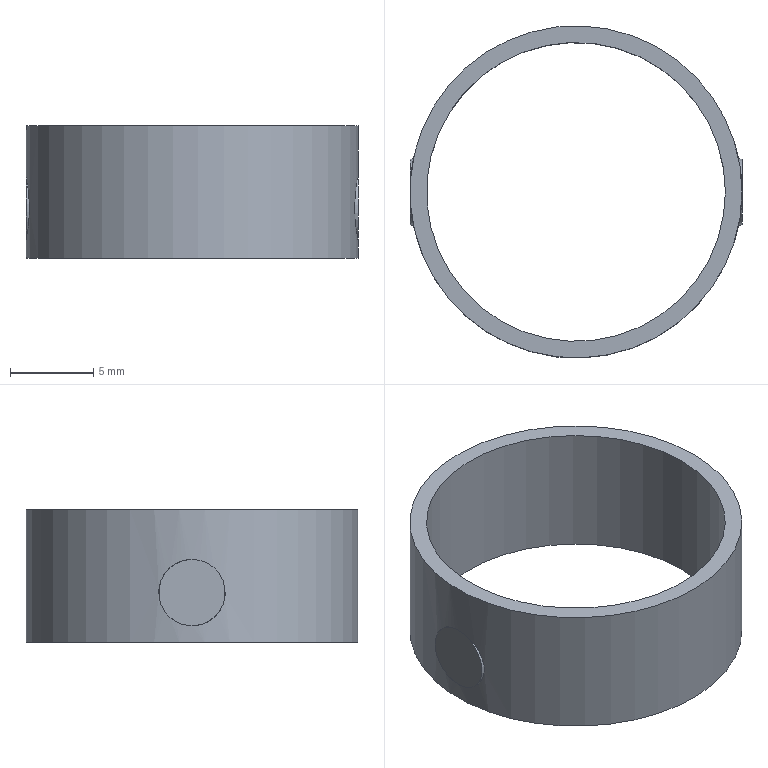Part | NX | features DATUM_CSYS 3, EXTRUDE 2, SKETCH 2, UNITE 2, Container 1, EXTRACT_BODY 1, Geometry Instance 1 | 1 solid | 10 faces | box 20 x 20 x 8 mm | volume 478.886 mm3 | cylinder 6 | plane 4 | commonest cylinder face diameters 4 x4 18 x1 20 x1
STEP:
#1=CARTESIAN_POINT('',(-10.,0.,1.));
#2=VERTEX_POINT('',#1);
#3=CARTESIAN_POINT('',(-10.,0.,5.));
#4=VERTEX_POINT('',#3);
#5=CARTESIAN_POINT('',(-10.,0.,1.));
#6=CARTESIAN_POINT('',(-10.,0.5227,1.));
#7=CARTESIAN_POINT('',(-9.9,1.565,1.432));
#8=CARTESIAN_POINT('',(-9.747,2.217,2.999));
#9=CARTESIAN_POINT('',(-9.9,1.565,4.566));
#10=CARTESIAN_POINT('',(-10.,0.5299,5.));
#11=CARTESIAN_POINT('',(-10.,0.,5.));
#12=B_SPLINE_CURVE_WITH_KNOTS('',3,(#5,#6,#7,#8,#9,#10,#11),.UNSPECIFIED.,.F.,.F.,(4,1,1,1,4),(0.006269,0.007836,0.009402,0.01097,0.01254),.UNSPECIFIED.);
#13=EDGE_CURVE('',#2,#4,#12,.T.);
#14=ORIENTED_EDGE('',*,*,#13,.F.);
#15=CARTESIAN_POINT('',(-10.,0.,3.));
#16=DIRECTION('',(1.,0.,0.));
#17=DIRECTION('',(0.,1.,0.));
#18=AXIS2_PLACEMENT_3D('',#15,#16,#17);
#19=CIRCLE('',#18,2.);
#20=EDGE_CURVE('',#4,#2,#19,.F.);
#21=ORIENTED_EDGE('',*,*,#20,.F.);
#22=EDGE_LOOP('',(#14,#21));
#23=FACE_BOUND('',#22,.T.);
#24=CARTESIAN_POINT('',(-10.,0.,3.));
#25=DIRECTION('',(1.,0.,0.));
#26=DIRECTION('',(0.,0.,1.));
#27=AXIS2_PLACEMENT_3D('',#24,#25,#26);
#28=CYLINDRICAL_SURFACE('',#27,2.);
#29=ADVANCED_FACE('',(#23),#28,.T.);
#30=CARTESIAN_POINT('',(-10.,0.,5.));
#31=CARTESIAN_POINT('',(-10.,-0.53,5.));
#32=CARTESIAN_POINT('',(-9.9,-1.564,4.566));
#33=CARTESIAN_POINT('',(-9.747,-2.217,3.002));
#34=CARTESIAN_POINT('',(-9.9,-1.567,1.432));
#35=CARTESIAN_POINT('',(-10.,-0.5228,1.));
#36=CARTESIAN_POINT('',(-10.,0.,1.));
#37=B_SPLINE_CURVE_WITH_KNOTS('',3,(#30,#31,#32,#33,#34,#35,#36),.UNSPECIFIED.,.F.,.F.,(4,1,1,1,4),(0.,0.001567,0.003134,0.004702,0.006269),.UNSPECIFIED.);
#38=EDGE_CURVE('',#4,#2,#37,.T.);
#39=ORIENTED_EDGE('',*,*,#38,.F.);
#40=CARTESIAN_POINT('',(-10.,0.,3.));
#41=DIRECTION('',(1.,0.,0.));
#42=DIRECTION('',(0.,1.,0.));
#43=AXIS2_PLACEMENT_3D('',#40,#41,#42);
#44=CIRCLE('',#43,2.);
#45=EDGE_CURVE('',#2,#4,#44,.F.);
#46=ORIENTED_EDGE('',*,*,#45,.F.);
#47=EDGE_LOOP('',(#39,#46));
#48=FACE_BOUND('',#47,.T.);
#49=CARTESIAN_POINT('',(-10.,0.,3.));
#50=DIRECTION('',(1.,0.,0.));
#51=DIRECTION('',(0.,0.,1.));
#52=AXIS2_PLACEMENT_3D('',#49,#50,#51);
#53=CYLINDRICAL_SURFACE('',#52,2.);
#54=ADVANCED_FACE('',(#48),#53,.T.);
#55=ORIENTED_EDGE('',*,*,#45,.T.);
#56=ORIENTED_EDGE('',*,*,#20,.T.);
#57=EDGE_LOOP('',(#55,#56));
#58=FACE_BOUND('',#57,.T.);
#59=CARTESIAN_POINT('',(-10.,0.,3.));
#60=DIRECTION('',(-1.,0.,0.));
#61=DIRECTION('',(0.,0.,-1.));
#62=AXIS2_PLACEMENT_3D('',#59,#60,#61);
#63=PLANE('',#62);
#64=ADVANCED_FACE('',(#58),#63,.T.);
#65=CARTESIAN_POINT('',(10.,0.,1.));
#66=VERTEX_POINT('',#65);
#67=CARTESIAN_POINT('',(10.,0.,5.));
#68=VERTEX_POINT('',#67);
#69=CARTESIAN_POINT('',(10.,0.,3.));
#70=DIRECTION('',(1.,0.,0.));
#71=DIRECTION('',(0.,1.,0.));
#72=AXIS2_PLACEMENT_3D('',#69,#70,#71);
#73=CIRCLE('',#72,2.);
#74=EDGE_CURVE('',#66,#68,#73,.T.);
#75=ORIENTED_EDGE('',*,*,#74,.T.);
#76=CARTESIAN_POINT('',(10.,0.,3.));
#77=DIRECTION('',(1.,0.,0.));
#78=DIRECTION('',(0.,1.,0.));
#79=AXIS2_PLACEMENT_3D('',#76,#77,#78);
#80=CIRCLE('',#79,2.);
#81=EDGE_CURVE('',#68,#66,#80,.T.);
#82=ORIENTED_EDGE('',*,*,#81,.T.);
#83=EDGE_LOOP('',(#75,#82));
#84=FACE_BOUND('',#83,.T.);
#85=CARTESIAN_POINT('',(10.,0.,3.));
#86=DIRECTION('',(1.,0.,0.));
#87=DIRECTION('',(0.,0.,-1.));
#88=AXIS2_PLACEMENT_3D('',#85,#86,#87);
#89=PLANE('',#88);
#90=ADVANCED_FACE('',(#84),#89,.T.);
#91=CARTESIAN_POINT('',(10.,0.,5.));
#92=CARTESIAN_POINT('',(10.,0.53,5.));
#93=CARTESIAN_POINT('',(9.9,1.564,4.566));
#94=CARTESIAN_POINT('',(9.747,2.217,3.002));
#95=CARTESIAN_POINT('',(9.9,1.567,1.432));
#96=CARTESIAN_POINT('',(10.,0.5228,1.));
#97=CARTESIAN_POINT('',(10.,0.,1.));
#98=B_SPLINE_CURVE_WITH_KNOTS('',3,(#91,#92,#93,#94,#95,#96,#97),.UNSPECIFIED.,.F.,.F.,(4,1,1,1,4),(0.,0.001567,0.003134,0.004702,0.006269),.UNSPECIFIED.);
#99=EDGE_CURVE('',#68,#66,#98,.T.);
#100=ORIENTED_EDGE('',*,*,#99,.F.);
#101=ORIENTED_EDGE('',*,*,#74,.F.);
#102=EDGE_LOOP('',(#100,#101));
#103=FACE_BOUND('',#102,.T.);
#104=CARTESIAN_POINT('',(10.,0.,3.));
#105=DIRECTION('',(-1.,0.,0.));
#106=DIRECTION('',(0.,0.,1.));
#107=AXIS2_PLACEMENT_3D('',#104,#105,#106);
#108=CYLINDRICAL_SURFACE('',#107,2.);
#109=ADVANCED_FACE('',(#103),#108,.T.);
#110=CARTESIAN_POINT('',(10.,0.,1.));
#111=CARTESIAN_POINT('',(10.,-0.5227,1.));
#112=CARTESIAN_POINT('',(9.9,-1.565,1.432));
#113=CARTESIAN_POINT('',(9.747,-2.217,2.999));
#114=CARTESIAN_POINT('',(9.9,-1.565,4.566));
#115=CARTESIAN_POINT('',(10.,-0.5299,5.));
#116=CARTESIAN_POINT('',(10.,0.,5.));
#117=B_SPLINE_CURVE_WITH_KNOTS('',3,(#110,#111,#112,#113,#114,#115,#116),.UNSPECIFIED.,.F.,.F.,(4,1,1,1,4),(0.006269,0.007836,0.009402,0.01097,0.01254),.UNSPECIFIED.);
#118=EDGE_CURVE('',#66,#68,#117,.T.);
#119=ORIENTED_EDGE('',*,*,#118,.F.);
#120=ORIENTED_EDGE('',*,*,#81,.F.);
#121=EDGE_LOOP('',(#119,#120));
#122=FACE_BOUND('',#121,.T.);
#123=CARTESIAN_POINT('',(10.,0.,3.));
#124=DIRECTION('',(-1.,0.,0.));
#125=DIRECTION('',(0.,0.,1.));
#126=AXIS2_PLACEMENT_3D('',#123,#124,#125);
#127=CYLINDRICAL_SURFACE('',#126,2.);
#128=ADVANCED_FACE('',(#122),#127,.T.);
#129=CARTESIAN_POINT('',(10.,0.,0.));
#130=VERTEX_POINT('',#129);
#131=CARTESIAN_POINT('',(0.,0.,0.));
#132=DIRECTION('',(0.,0.,1.));
#133=DIRECTION('',(1.,0.,0.));
#134=AXIS2_PLACEMENT_3D('',#131,#132,#133);
#135=CIRCLE('',#134,10.);
#136=EDGE_CURVE('',#130,#130,#135,.T.);
#137=ORIENTED_EDGE('',*,*,#136,.F.);
#138=EDGE_LOOP('',(#137));
#139=FACE_BOUND('',#138,.T.);
#140=CARTESIAN_POINT('',(9.,0.,0.));
#141=VERTEX_POINT('',#140);
#142=CARTESIAN_POINT('',(0.,0.,0.));
#143=DIRECTION('',(0.,0.,1.));
#144=DIRECTION('',(1.,0.,0.));
#145=AXIS2_PLACEMENT_3D('',#142,#143,#144);
#146=CIRCLE('',#145,9.);
#147=EDGE_CURVE('',#141,#141,#146,.T.);
#148=ORIENTED_EDGE('',*,*,#147,.T.);
#149=EDGE_LOOP('',(#148));
#150=FACE_BOUND('',#149,.T.);
#151=CARTESIAN_POINT('',(0.,0.,0.));
#152=DIRECTION('',(0.,0.,1.));
#153=DIRECTION('',(1.,0.,0.));
#154=AXIS2_PLACEMENT_3D('',#151,#152,#153);
#155=PLANE('',#154);
#156=ADVANCED_FACE('',(#139,#150),#155,.F.);
#157=CARTESIAN_POINT('',(10.,0.,8.));
#158=VERTEX_POINT('',#157);
#159=CARTESIAN_POINT('',(0.,0.,8.));
#160=DIRECTION('',(0.,0.,1.));
#161=DIRECTION('',(1.,0.,0.));
#162=AXIS2_PLACEMENT_3D('',#159,#160,#161);
#163=CIRCLE('',#162,10.);
#164=EDGE_CURVE('',#158,#158,#163,.T.);
#165=ORIENTED_EDGE('',*,*,#164,.T.);
#166=EDGE_LOOP('',(#165));
#167=FACE_BOUND('',#166,.T.);
#168=CARTESIAN_POINT('',(9.,0.,8.));
#169=VERTEX_POINT('',#168);
#170=CARTESIAN_POINT('',(0.,0.,8.));
#171=DIRECTION('',(0.,0.,1.));
#172=DIRECTION('',(1.,0.,0.));
#173=AXIS2_PLACEMENT_3D('',#170,#171,#172);
#174=CIRCLE('',#173,9.);
#175=EDGE_CURVE('',#169,#169,#174,.T.);
#176=ORIENTED_EDGE('',*,*,#175,.F.);
#177=EDGE_LOOP('',(#176));
#178=FACE_BOUND('',#177,.T.);
#179=CARTESIAN_POINT('',(0.,0.,8.));
#180=DIRECTION('',(0.,0.,1.));
#181=DIRECTION('',(1.,0.,0.));
#182=AXIS2_PLACEMENT_3D('',#179,#180,#181);
#183=PLANE('',#182);
#184=ADVANCED_FACE('',(#167,#178),#183,.T.);
#185=ORIENTED_EDGE('',*,*,#164,.F.);
#186=EDGE_LOOP('',(#185));
#187=FACE_BOUND('',#186,.T.);
#188=ORIENTED_EDGE('',*,*,#136,.T.);
#189=EDGE_LOOP('',(#188));
#190=FACE_BOUND('',#189,.T.);
#191=ORIENTED_EDGE('',*,*,#118,.T.);
#192=ORIENTED_EDGE('',*,*,#99,.T.);
#193=EDGE_LOOP('',(#191,#192));
#194=FACE_BOUND('',#193,.T.);
#195=ORIENTED_EDGE('',*,*,#13,.T.);
#196=ORIENTED_EDGE('',*,*,#38,.T.);
#197=EDGE_LOOP('',(#195,#196));
#198=FACE_BOUND('',#197,.T.);
#199=CARTESIAN_POINT('',(0.,0.,8.));
#200=DIRECTION('',(0.,0.,-1.));
#201=DIRECTION('',(-1.,0.,0.));
#202=AXIS2_PLACEMENT_3D('',#199,#200,#201);
#203=CYLINDRICAL_SURFACE('',#202,10.);
#204=ADVANCED_FACE('',(#187,#190,#194,#198),#203,.T.);
#205=ORIENTED_EDGE('',*,*,#175,.T.);
#206=EDGE_LOOP('',(#205));
#207=FACE_BOUND('',#206,.T.);
#208=ORIENTED_EDGE('',*,*,#147,.F.);
#209=EDGE_LOOP('',(#208));
#210=FACE_BOUND('',#209,.T.);
#211=CARTESIAN_POINT('',(0.,0.,8.));
#212=DIRECTION('',(0.,0.,-1.));
#213=DIRECTION('',(-1.,0.,0.));
#214=AXIS2_PLACEMENT_3D('',#211,#212,#213);
#215=CYLINDRICAL_SURFACE('',#214,9.);
#216=ADVANCED_FACE('',(#207,#210),#215,.F.);
#217=CLOSED_SHELL('',(#29,#54,#64,#90,#109,#128,#156,#184,#204,#216));
#218=MANIFOLD_SOLID_BREP('',#217);
#219=(LENGTH_UNIT()NAMED_UNIT(*)SI_UNIT(.MILLI.,.METRE.));
#220=UNCERTAINTY_MEASURE_WITH_UNIT(LENGTH_MEASURE(0.0508),#219,'','');
#221=(NAMED_UNIT(*)PLANE_ANGLE_UNIT()SI_UNIT($,.RADIAN.));
#222=(NAMED_UNIT(*)SI_UNIT($,.STERADIAN.)SOLID_ANGLE_UNIT());
#223=(GEOMETRIC_REPRESENTATION_CONTEXT(3)GLOBAL_UNCERTAINTY_ASSIGNED_CONTEXT((#220))GLOBAL_UNIT_ASSIGNED_CONTEXT((#219,#221,#222))REPRESENTATION_CONTEXT('',''));
#224=ADVANCED_BREP_SHAPE_REPRESENTATION('',(#218),#223);